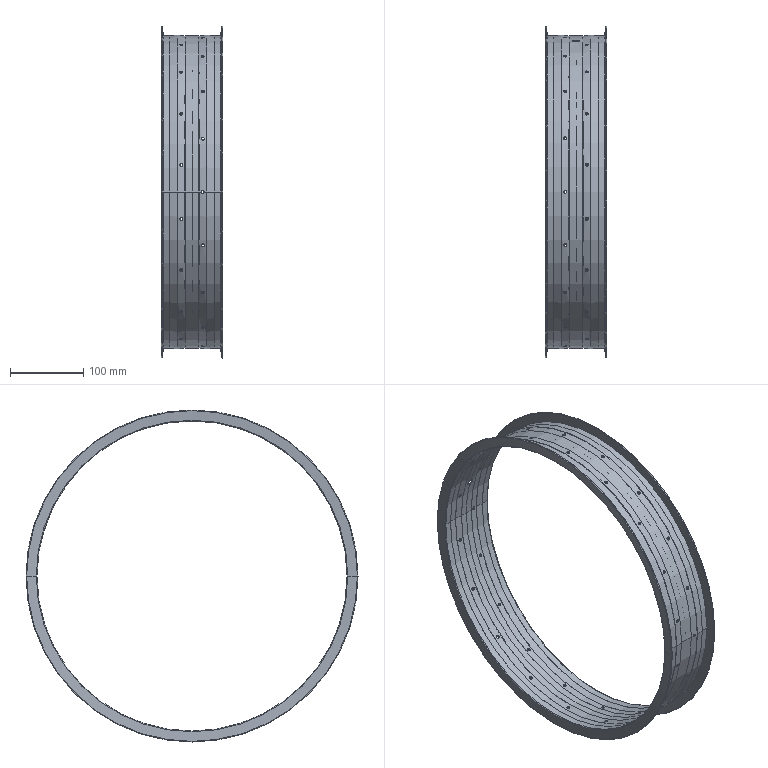Part | STEP file | BREP_1 | 1 solid | 136 faces | box 83.255 x 451.856 x 451.856 mm | volume 216324 mm3 | cylinder 88 | cone 24 | torus 24 | commonest cylinder face diameters 4 x72 421.997 x8 425 x6 9 x2